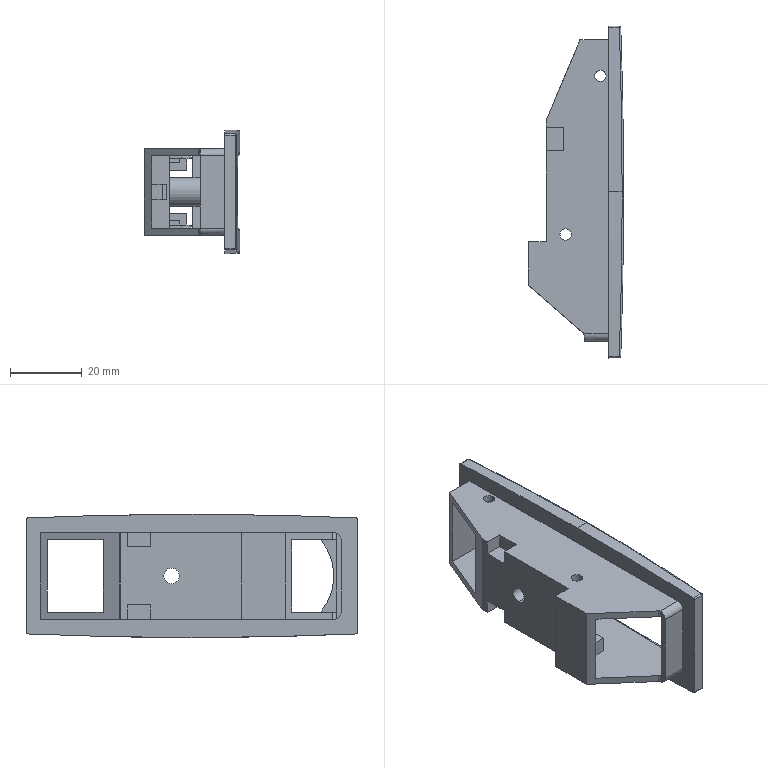Part | SolidWorks | features BaseBody 1 | 1 solid | 95 faces | box 26.6 x 92.8 x 34.425 mm | volume 14657 mm3 | plane 51 | cylinder 34 | spline 6 | sphere 4 | commonest cylinder face diameters 3.2 x8 0.8 x6 5.436 x4 1.6 x2 2.6 x2 4 x2